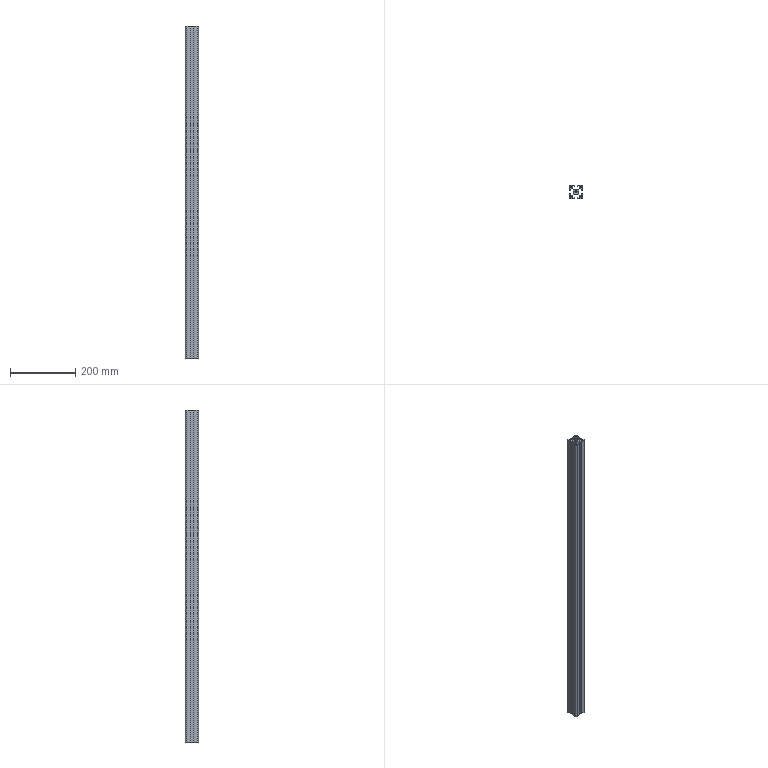Part | NX | features DATUM_CSYS 2, EXTRUDE 1, SKETCH 1 | 1 solid | 103 faces | box 40 x 40 x 1020 mm | volume 588076 mm3 | plane 94 | cylinder 9 | commonest cylinder face diameters 5 x4 9 x4 6.8 x1